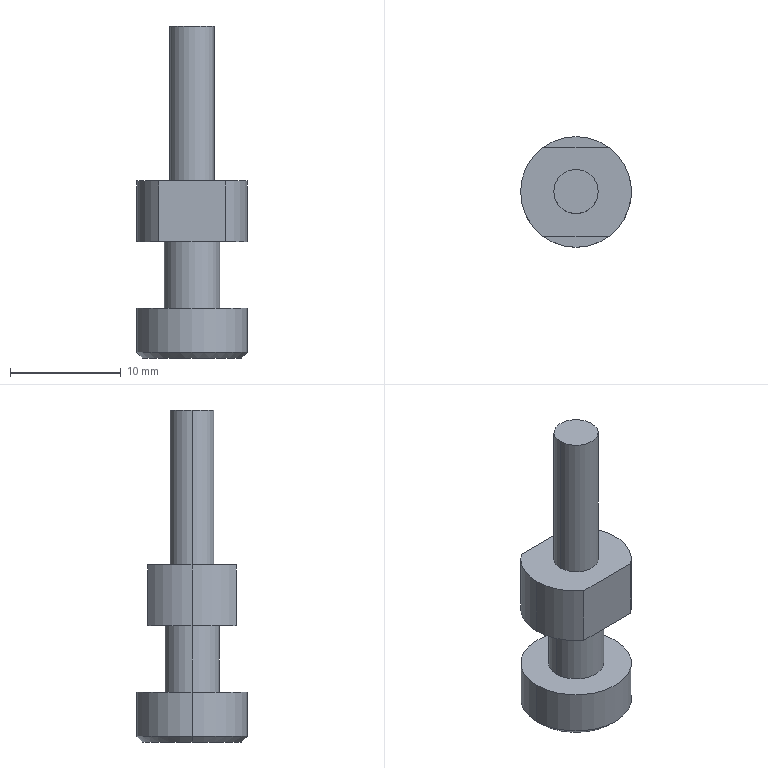Part | STEP file | PN_0008 Mount electronic clip movable head A | 1 solid | 18 faces | box 10 x 10 x 30 mm | volume 1030 mm3 | cylinder 9 | plane 7 | cone 2 | commonest cylinder face diameters 10 x5 4 x2 5 x2
STEP:
#1=CARTESIAN_POINT('',(0.,0.,0.));
#2=DIRECTION('',(0.,0.,1.));
#3=DIRECTION('',(1.,0.,0.));
#4=AXIS2_PLACEMENT_3D('',#1,#2,#3);
#5=CARTESIAN_POINT('',(-4.5,0.,-10.5));
#6=VERTEX_POINT('',#5);
#7=CARTESIAN_POINT('',(4.5,0.,-10.5));
#8=VERTEX_POINT('',#7);
#9=CARTESIAN_POINT('',(0.,0.,-10.5));
#10=DIRECTION('',(0.,0.,-1.));
#11=DIRECTION('',(-1.,0.,0.));
#12=AXIS2_PLACEMENT_3D('',#9,#10,#11);
#13=CIRCLE('',#12,4.5);
#14=CARTESIAN_POINT('',(0.,0.,-10.5));
#15=DIRECTION('',(0.,0.,1.));
#16=DIRECTION('',(1.,0.,0.));
#17=AXIS2_PLACEMENT_3D('',#14,#15,#16);
#18=CONICAL_SURFACE('',#17,4.5,0.7854);
#19=CARTESIAN_POINT('',(3.142,0.));
#20=DIRECTION('',(-1.,0.));
#21=VECTOR('',#20,1.);
#22=LINE('',#19,#21);
#23=(GEOMETRIC_REPRESENTATION_CONTEXT(2)PARAMETRIC_REPRESENTATION_CONTEXT()REPRESENTATION_CONTEXT('',''));
#24=DEFINITIONAL_REPRESENTATION('',(#22),#23);
#25=PCURVE('',#18,#24);
#26=CARTESIAN_POINT('',(0.,0.,-10.5));
#27=DIRECTION('',(0.,0.,-1.));
#28=DIRECTION('',(-1.,0.,0.));
#29=AXIS2_PLACEMENT_3D('',#26,#27,#28);
#30=PLANE('',#29);
#31=CARTESIAN_POINT('',(0.,0.));
#32=DIRECTION('',(1.,0.));
#33=AXIS2_PLACEMENT_2D('',#31,#32);
#34=CIRCLE('',#33,4.5);
#35=(GEOMETRIC_REPRESENTATION_CONTEXT(2)PARAMETRIC_REPRESENTATION_CONTEXT()REPRESENTATION_CONTEXT('',''));
#36=DEFINITIONAL_REPRESENTATION('',(#34),#35);
#37=PCURVE('',#30,#36);
#38=SURFACE_CURVE('',#13,(#25,#37),.PCURVE_S1.);
#39=EDGE_CURVE('',#6,#8,#38,.T.);
#40=ORIENTED_EDGE('',*,*,#39,.F.);
#41=CARTESIAN_POINT('',(-5.,0.,-10.));
#42=VERTEX_POINT('',#41);
#43=CARTESIAN_POINT('',(-4.5,0.,-10.5));
#44=DIRECTION('',(-0.7071,0.,0.7071));
#45=VECTOR('',#44,1.);
#46=LINE('',#43,#45);
#47=CARTESIAN_POINT('',(3.142,0.));
#48=DIRECTION('',(0.,1.));
#49=VECTOR('',#48,1.);
#50=LINE('',#47,#49);
#51=(GEOMETRIC_REPRESENTATION_CONTEXT(2)PARAMETRIC_REPRESENTATION_CONTEXT()REPRESENTATION_CONTEXT('',''));
#52=DEFINITIONAL_REPRESENTATION('',(#50),#51);
#53=PCURVE('',#18,#52);
#54=CARTESIAN_POINT('',(0.,0.,-10.5));
#55=DIRECTION('',(0.,0.,1.));
#56=DIRECTION('',(1.,0.,0.));
#57=AXIS2_PLACEMENT_3D('',#54,#55,#56);
#58=CONICAL_SURFACE('',#57,4.5,0.7854);
#59=CARTESIAN_POINT('',(3.142,0.));
#60=DIRECTION('',(0.,1.));
#61=VECTOR('',#60,1.);
#62=LINE('',#59,#61);
#63=(GEOMETRIC_REPRESENTATION_CONTEXT(2)PARAMETRIC_REPRESENTATION_CONTEXT()REPRESENTATION_CONTEXT('',''));
#64=DEFINITIONAL_REPRESENTATION('',(#62),#63);
#65=PCURVE('',#58,#64);
#66=SURFACE_CURVE('',#46,(#53,#65),.PCURVE_S1.);
#67=EDGE_CURVE('',#6,#42,#66,.T.);
#68=ORIENTED_EDGE('',*,*,#67,.T.);
#69=CARTESIAN_POINT('',(5.,0.,-10.));
#70=VERTEX_POINT('',#69);
#71=CARTESIAN_POINT('',(0.,0.,-10.));
#72=DIRECTION('',(0.,0.,1.));
#73=DIRECTION('',(-1.,0.,0.));
#74=AXIS2_PLACEMENT_3D('',#71,#72,#73);
#75=CIRCLE('',#74,5.);
#76=CARTESIAN_POINT('',(-3.142,0.5));
#77=DIRECTION('',(1.,0.));
#78=VECTOR('',#77,1.);
#79=LINE('',#76,#78);
#80=(GEOMETRIC_REPRESENTATION_CONTEXT(2)PARAMETRIC_REPRESENTATION_CONTEXT()REPRESENTATION_CONTEXT('',''));
#81=DEFINITIONAL_REPRESENTATION('',(#79),#80);
#82=PCURVE('',#18,#81);
#83=CARTESIAN_POINT('',(0.,0.,-10.5));
#84=DIRECTION('',(0.,0.,1.));
#85=DIRECTION('',(1.,0.,0.));
#86=AXIS2_PLACEMENT_3D('',#83,#84,#85);
#87=CYLINDRICAL_SURFACE('',#86,5.);
#88=CARTESIAN_POINT('',(-3.142,0.5));
#89=DIRECTION('',(1.,0.));
#90=VECTOR('',#89,1.);
#91=LINE('',#88,#90);
#92=(GEOMETRIC_REPRESENTATION_CONTEXT(2)PARAMETRIC_REPRESENTATION_CONTEXT()REPRESENTATION_CONTEXT('',''));
#93=DEFINITIONAL_REPRESENTATION('',(#91),#92);
#94=PCURVE('',#87,#93);
#95=SURFACE_CURVE('',#75,(#82,#94),.PCURVE_S1.);
#96=EDGE_CURVE('',#70,#42,#95,.T.);
#97=ORIENTED_EDGE('',*,*,#96,.F.);
#98=CARTESIAN_POINT('',(4.5,0.,-10.5));
#99=DIRECTION('',(0.7071,0.,0.7071));
#100=VECTOR('',#99,1.);
#101=LINE('',#98,#100);
#102=CARTESIAN_POINT('',(0.,0.));
#103=DIRECTION('',(0.,1.));
#104=VECTOR('',#103,1.);
#105=LINE('',#102,#104);
#106=(GEOMETRIC_REPRESENTATION_CONTEXT(2)PARAMETRIC_REPRESENTATION_CONTEXT()REPRESENTATION_CONTEXT('',''));
#107=DEFINITIONAL_REPRESENTATION('',(#105),#106);
#108=PCURVE('',#18,#107);
#109=CARTESIAN_POINT('',(6.283,0.));
#110=DIRECTION('',(0.,1.));
#111=VECTOR('',#110,1.);
#112=LINE('',#109,#111);
#113=(GEOMETRIC_REPRESENTATION_CONTEXT(2)PARAMETRIC_REPRESENTATION_CONTEXT()REPRESENTATION_CONTEXT('',''));
#114=DEFINITIONAL_REPRESENTATION('',(#112),#113);
#115=PCURVE('',#58,#114);
#116=SURFACE_CURVE('',#101,(#108,#115),.PCURVE_S1.);
#117=EDGE_CURVE('',#8,#70,#116,.T.);
#118=ORIENTED_EDGE('',*,*,#117,.F.);
#119=EDGE_LOOP('',(#40,#68,#97,#118));
#120=FACE_BOUND('',#119,.T.);
#121=ADVANCED_FACE('',(#120),#18,.T.);
#122=ORIENTED_EDGE('',*,*,#96,.T.);
#123=CARTESIAN_POINT('',(-5.,0.,-6.));
#124=VERTEX_POINT('',#123);
#125=CARTESIAN_POINT('',(-5.,0.,-10.5));
#126=DIRECTION('',(0.,0.,1.));
#127=VECTOR('',#126,1.);
#128=LINE('',#125,#127);
#129=CARTESIAN_POINT('',(3.142,0.));
#130=DIRECTION('',(0.,1.));
#131=VECTOR('',#130,1.);
#132=LINE('',#129,#131);
#133=(GEOMETRIC_REPRESENTATION_CONTEXT(2)PARAMETRIC_REPRESENTATION_CONTEXT()REPRESENTATION_CONTEXT('',''));
#134=DEFINITIONAL_REPRESENTATION('',(#132),#133);
#135=PCURVE('',#87,#134);
#136=CARTESIAN_POINT('',(0.,0.,-10.5));
#137=DIRECTION('',(0.,0.,1.));
#138=DIRECTION('',(1.,0.,0.));
#139=AXIS2_PLACEMENT_3D('',#136,#137,#138);
#140=CYLINDRICAL_SURFACE('',#139,5.);
#141=CARTESIAN_POINT('',(3.142,0.));
#142=DIRECTION('',(0.,1.));
#143=VECTOR('',#142,1.);
#144=LINE('',#141,#143);
#145=(GEOMETRIC_REPRESENTATION_CONTEXT(2)PARAMETRIC_REPRESENTATION_CONTEXT()REPRESENTATION_CONTEXT('',''));
#146=DEFINITIONAL_REPRESENTATION('',(#144),#145);
#147=PCURVE('',#140,#146);
#148=SURFACE_CURVE('',#128,(#135,#147),.PCURVE_S1.);
#149=EDGE_CURVE('',#42,#124,#148,.T.);
#150=ORIENTED_EDGE('',*,*,#149,.T.);
#151=CARTESIAN_POINT('',(5.,0.,-6.));
#152=VERTEX_POINT('',#151);
#153=CARTESIAN_POINT('',(0.,0.,-6.));
#154=DIRECTION('',(0.,0.,-1.));
#155=DIRECTION('',(-1.,0.,0.));
#156=AXIS2_PLACEMENT_3D('',#153,#154,#155);
#157=CIRCLE('',#156,5.);
#158=CARTESIAN_POINT('',(3.142,4.5));
#159=DIRECTION('',(-1.,0.));
#160=VECTOR('',#159,1.);
#161=LINE('',#158,#160);
#162=(GEOMETRIC_REPRESENTATION_CONTEXT(2)PARAMETRIC_REPRESENTATION_CONTEXT()REPRESENTATION_CONTEXT('',''));
#163=DEFINITIONAL_REPRESENTATION('',(#161),#162);
#164=PCURVE('',#87,#163);
#165=CARTESIAN_POINT('',(0.,0.,-6.));
#166=DIRECTION('',(0.,0.,-1.));
#167=DIRECTION('',(-1.,0.,0.));
#168=AXIS2_PLACEMENT_3D('',#165,#166,#167);
#169=PLANE('',#168);
#170=CARTESIAN_POINT('',(0.,0.));
#171=DIRECTION('',(1.,0.));
#172=AXIS2_PLACEMENT_2D('',#170,#171);
#173=CIRCLE('',#172,5.);
#174=(GEOMETRIC_REPRESENTATION_CONTEXT(2)PARAMETRIC_REPRESENTATION_CONTEXT()REPRESENTATION_CONTEXT('',''));
#175=DEFINITIONAL_REPRESENTATION('',(#173),#174);
#176=PCURVE('',#169,#175);
#177=SURFACE_CURVE('',#157,(#164,#176),.PCURVE_S1.);
#178=EDGE_CURVE('',#124,#152,#177,.T.);
#179=ORIENTED_EDGE('',*,*,#178,.T.);
#180=CARTESIAN_POINT('',(5.,0.,-10.5));
#181=DIRECTION('',(0.,0.,1.));
#182=VECTOR('',#181,1.);
#183=LINE('',#180,#182);
#184=CARTESIAN_POINT('',(0.,0.));
#185=DIRECTION('',(0.,1.));
#186=VECTOR('',#185,1.);
#187=LINE('',#184,#186);
#188=(GEOMETRIC_REPRESENTATION_CONTEXT(2)PARAMETRIC_REPRESENTATION_CONTEXT()REPRESENTATION_CONTEXT('',''));
#189=DEFINITIONAL_REPRESENTATION('',(#187),#188);
#190=PCURVE('',#87,#189);
#191=CARTESIAN_POINT('',(6.283,0.));
#192=DIRECTION('',(0.,1.));
#193=VECTOR('',#192,1.);
#194=LINE('',#191,#193);
#195=(GEOMETRIC_REPRESENTATION_CONTEXT(2)PARAMETRIC_REPRESENTATION_CONTEXT()REPRESENTATION_CONTEXT('',''));
#196=DEFINITIONAL_REPRESENTATION('',(#194),#195);
#197=PCURVE('',#140,#196);
#198=SURFACE_CURVE('',#183,(#190,#197),.PCURVE_S1.);
#199=EDGE_CURVE('',#70,#152,#198,.T.);
#200=ORIENTED_EDGE('',*,*,#199,.F.);
#201=EDGE_LOOP('',(#122,#150,#179,#200));
#202=FACE_BOUND('',#201,.T.);
#203=ADVANCED_FACE('',(#202),#87,.T.);
#204=CARTESIAN_POINT('',(-2.5,0.,-6.));
#205=VERTEX_POINT('',#204);
#206=CARTESIAN_POINT('',(2.5,0.,-6.));
#207=VERTEX_POINT('',#206);
#208=CARTESIAN_POINT('',(0.,0.,-6.));
#209=DIRECTION('',(0.,0.,-1.));
#210=DIRECTION('',(-1.,0.,0.));
#211=AXIS2_PLACEMENT_3D('',#208,#209,#210);
#212=CIRCLE('',#211,2.5);
#213=CARTESIAN_POINT('',(0.,0.,-6.));
#214=DIRECTION('',(0.,0.,1.));
#215=DIRECTION('',(1.,0.,0.));
#216=AXIS2_PLACEMENT_3D('',#213,#214,#215);
#217=CYLINDRICAL_SURFACE('',#216,2.5);
#218=CARTESIAN_POINT('',(3.142,0.));
#219=DIRECTION('',(-1.,0.));
#220=VECTOR('',#219,1.);
#221=LINE('',#218,#220);
#222=(GEOMETRIC_REPRESENTATION_CONTEXT(2)PARAMETRIC_REPRESENTATION_CONTEXT()REPRESENTATION_CONTEXT('',''));
#223=DEFINITIONAL_REPRESENTATION('',(#221),#222);
#224=PCURVE('',#217,#223);
#225=CARTESIAN_POINT('',(0.,0.));
#226=DIRECTION('',(1.,0.));
#227=AXIS2_PLACEMENT_2D('',#225,#226);
#228=CIRCLE('',#227,2.5);
#229=(GEOMETRIC_REPRESENTATION_CONTEXT(2)PARAMETRIC_REPRESENTATION_CONTEXT()REPRESENTATION_CONTEXT('',''));
#230=DEFINITIONAL_REPRESENTATION('',(#228),#229);
#231=PCURVE('',#169,#230);
#232=SURFACE_CURVE('',#212,(#224,#231),.PCURVE_S1.);
#233=EDGE_CURVE('',#205,#207,#232,.T.);
#234=ORIENTED_EDGE('',*,*,#233,.F.);
#235=CARTESIAN_POINT('',(-2.5,0.,0.));
#236=VERTEX_POINT('',#235);
#237=CARTESIAN_POINT('',(-2.5,0.,-6.));
#238=DIRECTION('',(0.,0.,1.));
#239=VECTOR('',#238,1.);
#240=LINE('',#237,#239);
#241=CARTESIAN_POINT('',(3.142,0.));
#242=DIRECTION('',(0.,1.));
#243=VECTOR('',#242,1.);
#244=LINE('',#241,#243);
#245=(GEOMETRIC_REPRESENTATION_CONTEXT(2)PARAMETRIC_REPRESENTATION_CONTEXT()REPRESENTATION_CONTEXT('',''));
#246=DEFINITIONAL_REPRESENTATION('',(#244),#245);
#247=PCURVE('',#217,#246);
#248=CARTESIAN_POINT('',(0.,0.,-6.));
#249=DIRECTION('',(0.,0.,1.));
#250=DIRECTION('',(1.,0.,0.));
#251=AXIS2_PLACEMENT_3D('',#248,#249,#250);
#252=CYLINDRICAL_SURFACE('',#251,2.5);
#253=CARTESIAN_POINT('',(3.142,0.));
#254=DIRECTION('',(0.,1.));
#255=VECTOR('',#254,1.);
#256=LINE('',#253,#255);
#257=(GEOMETRIC_REPRESENTATION_CONTEXT(2)PARAMETRIC_REPRESENTATION_CONTEXT()REPRESENTATION_CONTEXT('',''));
#258=DEFINITIONAL_REPRESENTATION('',(#256),#257);
#259=PCURVE('',#252,#258);
#260=SURFACE_CURVE('',#240,(#247,#259),.PCURVE_S1.);
#261=EDGE_CURVE('',#205,#236,#260,.T.);
#262=ORIENTED_EDGE('',*,*,#261,.T.);
#263=CARTESIAN_POINT('',(2.5,0.,0.));
#264=VERTEX_POINT('',#263);
#265=CARTESIAN_POINT('',(0.,0.,0.));
#266=DIRECTION('',(0.,0.,-1.));
#267=DIRECTION('',(1.,0.,0.));
#268=AXIS2_PLACEMENT_3D('',#265,#266,#267);
#269=CIRCLE('',#268,2.5);
#270=CARTESIAN_POINT('',(6.283,6.));
#271=DIRECTION('',(-1.,0.));
#272=VECTOR('',#271,1.);
#273=LINE('',#270,#272);
#274=(GEOMETRIC_REPRESENTATION_CONTEXT(2)PARAMETRIC_REPRESENTATION_CONTEXT()REPRESENTATION_CONTEXT('',''));
#275=DEFINITIONAL_REPRESENTATION('',(#273),#274);
#276=PCURVE('',#217,#275);
#277=CARTESIAN_POINT('',(0.,0.,0.));
#278=DIRECTION('',(0.,0.,1.));
#279=DIRECTION('',(1.,0.,0.));
#280=AXIS2_PLACEMENT_3D('',#277,#278,#279);
#281=PLANE('',#280);
#282=CARTESIAN_POINT('',(2.5,0.));
#283=CARTESIAN_POINT('',(2.5,-4.33));
#284=CARTESIAN_POINT('',(-1.25,-2.165));
#285=CARTESIAN_POINT('',(-5.,0.));
#286=CARTESIAN_POINT('',(-1.25,2.165));
#287=CARTESIAN_POINT('',(2.5,4.33));
#288=CARTESIAN_POINT('',(2.5,0.));
#289=(BOUNDED_CURVE()B_SPLINE_CURVE(2,(#282,#283,#284,#285,#286,#287,#288),.UNSPECIFIED.,.T.,.F.)B_SPLINE_CURVE_WITH_KNOTS((1,2,2,2,2,1),(-2.094,0.,2.094,4.189,6.283,8.378),.UNSPECIFIED.)CURVE()GEOMETRIC_REPRESENTATION_ITEM()RATIONAL_B_SPLINE_CURVE((1.,0.5,1.,0.5,1.,0.5,1.))REPRESENTATION_ITEM(''));
#290=(GEOMETRIC_REPRESENTATION_CONTEXT(2)PARAMETRIC_REPRESENTATION_CONTEXT()REPRESENTATION_CONTEXT('',''));
#291=DEFINITIONAL_REPRESENTATION('',(#289),#290);
#292=PCURVE('',#281,#291);
#293=SURFACE_CURVE('',#269,(#276,#292),.PCURVE_S1.);
#294=EDGE_CURVE('',#236,#264,#293,.T.);
#295=ORIENTED_EDGE('',*,*,#294,.T.);
#296=CARTESIAN_POINT('',(2.5,0.,-6.));
#297=DIRECTION('',(0.,0.,1.));
#298=VECTOR('',#297,1.);
#299=LINE('',#296,#298);
#300=CARTESIAN_POINT('',(0.,0.));
#301=DIRECTION('',(0.,1.));
#302=VECTOR('',#301,1.);
#303=LINE('',#300,#302);
#304=(GEOMETRIC_REPRESENTATION_CONTEXT(2)PARAMETRIC_REPRESENTATION_CONTEXT()REPRESENTATION_CONTEXT('',''));
#305=DEFINITIONAL_REPRESENTATION('',(#303),#304);
#306=PCURVE('',#217,#305);
#307=CARTESIAN_POINT('',(6.283,0.));
#308=DIRECTION('',(0.,1.));
#309=VECTOR('',#308,1.);
#310=LINE('',#307,#309);
#311=(GEOMETRIC_REPRESENTATION_CONTEXT(2)PARAMETRIC_REPRESENTATION_CONTEXT()REPRESENTATION_CONTEXT('',''));
#312=DEFINITIONAL_REPRESENTATION('',(#310),#311);
#313=PCURVE('',#252,#312);
#314=SURFACE_CURVE('',#299,(#306,#313),.PCURVE_S1.);
#315=EDGE_CURVE('',#207,#264,#314,.T.);
#316=ORIENTED_EDGE('',*,*,#315,.F.);
#317=EDGE_LOOP('',(#234,#262,#295,#316));
#318=FACE_BOUND('',#317,.T.);
#319=ADVANCED_FACE('',(#318),#217,.T.);
#320=CARTESIAN_POINT('',(2.,0.,19.5));
#321=VERTEX_POINT('',#320);
#322=CARTESIAN_POINT('',(-2.,0.,19.5));
#323=VERTEX_POINT('',#322);
#324=CARTESIAN_POINT('',(0.,0.,19.5));
#325=DIRECTION('',(0.,0.,1.));
#326=DIRECTION('',(1.,0.,0.));
#327=AXIS2_PLACEMENT_3D('',#324,#325,#326);
#328=CIRCLE('',#327,2.);
#329=CARTESIAN_POINT('',(0.,0.,19.5));
#330=DIRECTION('',(0.,0.,-1.));
#331=DIRECTION('',(-1.,0.,0.));
#332=AXIS2_PLACEMENT_3D('',#329,#330,#331);
#333=CYLINDRICAL_SURFACE('',#332,2.);
#334=CARTESIAN_POINT('',(3.142,0.));
#335=DIRECTION('',(-1.,0.));
#336=VECTOR('',#335,1.);
#337=LINE('',#334,#336);
#338=(GEOMETRIC_REPRESENTATION_CONTEXT(2)PARAMETRIC_REPRESENTATION_CONTEXT()REPRESENTATION_CONTEXT('',''));
#339=DEFINITIONAL_REPRESENTATION('',(#337),#338);
#340=PCURVE('',#333,#339);
#341=CARTESIAN_POINT('',(0.,0.,19.5));
#342=DIRECTION('',(0.,0.,1.));
#343=DIRECTION('',(1.,0.,0.));
#344=AXIS2_PLACEMENT_3D('',#341,#342,#343);
#345=PLANE('',#344);
#346=CARTESIAN_POINT('',(0.,0.));
#347=DIRECTION('',(1.,0.));
#348=AXIS2_PLACEMENT_2D('',#346,#347);
#349=CIRCLE('',#348,2.);
#350=(GEOMETRIC_REPRESENTATION_CONTEXT(2)PARAMETRIC_REPRESENTATION_CONTEXT()REPRESENTATION_CONTEXT('',''));
#351=DEFINITIONAL_REPRESENTATION('',(#349),#350);
#352=PCURVE('',#345,#351);
#353=SURFACE_CURVE('',#328,(#340,#352),.PCURVE_S1.);
#354=EDGE_CURVE('',#321,#323,#353,.T.);
#355=ORIENTED_EDGE('',*,*,#354,.F.);
#356=CARTESIAN_POINT('',(2.,0.,5.5));
#357=VERTEX_POINT('',#356);
#358=CARTESIAN_POINT('',(2.,0.,19.5));
#359=DIRECTION('',(0.,0.,-1.));
#360=VECTOR('',#359,1.);
#361=LINE('',#358,#360);
#362=CARTESIAN_POINT('',(3.142,0.));
#363=DIRECTION('',(0.,1.));
#364=VECTOR('',#363,1.);
#365=LINE('',#362,#364);
#366=(GEOMETRIC_REPRESENTATION_CONTEXT(2)PARAMETRIC_REPRESENTATION_CONTEXT()REPRESENTATION_CONTEXT('',''));
#367=DEFINITIONAL_REPRESENTATION('',(#365),#366);
#368=PCURVE('',#333,#367);
#369=CARTESIAN_POINT('',(0.,0.,19.5));
#370=DIRECTION('',(0.,0.,-1.));
#371=DIRECTION('',(-1.,0.,0.));
#372=AXIS2_PLACEMENT_3D('',#369,#370,#371);
#373=CYLINDRICAL_SURFACE('',#372,2.);
#374=CARTESIAN_POINT('',(3.142,0.));
#375=DIRECTION('',(0.,1.));
#376=VECTOR('',#375,1.);
#377=LINE('',#374,#376);
#378=(GEOMETRIC_REPRESENTATION_CONTEXT(2)PARAMETRIC_REPRESENTATION_CONTEXT()REPRESENTATION_CONTEXT('',''));
#379=DEFINITIONAL_REPRESENTATION('',(#377),#378);
#380=PCURVE('',#373,#379);
#381=SURFACE_CURVE('',#361,(#368,#380),.PCURVE_S1.);
#382=EDGE_CURVE('',#321,#357,#381,.T.);
#383=ORIENTED_EDGE('',*,*,#382,.T.);
#384=CARTESIAN_POINT('',(-2.,0.,5.5));
#385=VERTEX_POINT('',#384);
#386=CARTESIAN_POINT('',(0.,0.,5.5));
#387=DIRECTION('',(0.,0.,1.));
#388=DIRECTION('',(1.,0.,0.));
#389=AXIS2_PLACEMENT_3D('',#386,#387,#388);
#390=CIRCLE('',#389,2.);
#391=CARTESIAN_POINT('',(3.142,14.));
#392=DIRECTION('',(-1.,0.));
#393=VECTOR('',#392,1.);
#394=LINE('',#391,#393);
#395=(GEOMETRIC_REPRESENTATION_CONTEXT(2)PARAMETRIC_REPRESENTATION_CONTEXT()REPRESENTATION_CONTEXT('',''));
#396=DEFINITIONAL_REPRESENTATION('',(#394),#395);
#397=PCURVE('',#333,#396);
#398=CARTESIAN_POINT('',(0.,0.,5.5));
#399=DIRECTION('',(0.,0.,1.));
#400=DIRECTION('',(1.,0.,0.));
#401=AXIS2_PLACEMENT_3D('',#398,#399,#400);
#402=PLANE('',#401);
#403=CARTESIAN_POINT('',(0.,0.));
#404=DIRECTION('',(1.,0.));
#405=AXIS2_PLACEMENT_2D('',#403,#404);
#406=CIRCLE('',#405,2.);
#407=(GEOMETRIC_REPRESENTATION_CONTEXT(2)PARAMETRIC_REPRESENTATION_CONTEXT()REPRESENTATION_CONTEXT('',''));
#408=DEFINITIONAL_REPRESENTATION('',(#406),#407);
#409=PCURVE('',#402,#408);
#410=SURFACE_CURVE('',#390,(#397,#409),.PCURVE_S1.);
#411=EDGE_CURVE('',#357,#385,#410,.T.);
#412=ORIENTED_EDGE('',*,*,#411,.T.);
#413=CARTESIAN_POINT('',(-2.,0.,19.5));
#414=DIRECTION('',(0.,0.,-1.));
#415=VECTOR('',#414,1.);
#416=LINE('',#413,#415);
#417=CARTESIAN_POINT('',(0.,0.));
#418=DIRECTION('',(0.,1.));
#419=VECTOR('',#418,1.);
#420=LINE('',#417,#419);
#421=(GEOMETRIC_REPRESENTATION_CONTEXT(2)PARAMETRIC_REPRESENTATION_CONTEXT()REPRESENTATION_CONTEXT('',''));
#422=DEFINITIONAL_REPRESENTATION('',(#420),#421);
#423=PCURVE('',#333,#422);
#424=CARTESIAN_POINT('',(6.283,0.));
#425=DIRECTION('',(0.,1.));
#426=VECTOR('',#425,1.);
#427=LINE('',#424,#426);
#428=(GEOMETRIC_REPRESENTATION_CONTEXT(2)PARAMETRIC_REPRESENTATION_CONTEXT()REPRESENTATION_CONTEXT('',''));
#429=DEFINITIONAL_REPRESENTATION('',(#427),#428);
#430=PCURVE('',#373,#429);
#431=SURFACE_CURVE('',#416,(#423,#430),.PCURVE_S1.);
#432=EDGE_CURVE('',#323,#385,#431,.T.);
#433=ORIENTED_EDGE('',*,*,#432,.F.);
#434=EDGE_LOOP('',(#355,#383,#412,#433));
#435=FACE_BOUND('',#434,.T.);
#436=ADVANCED_FACE('',(#435),#333,.T.);
#437=CARTESIAN_POINT('',(-5.,0.,5.5));
#438=VERTEX_POINT('',#437);
#439=CARTESIAN_POINT('',(-3.,-4.,5.5));
#440=VERTEX_POINT('',#439);
#441=CARTESIAN_POINT('',(0.,0.,5.5));
#442=DIRECTION('',(0.,0.,1.));
#443=DIRECTION('',(1.,0.,0.));
#444=AXIS2_PLACEMENT_3D('',#441,#442,#443);
#445=CIRCLE('',#444,5.);
#446=CARTESIAN_POINT('',(0.,0.,5.5));
#447=DIRECTION('',(0.,0.,-1.));
#448=DIRECTION('',(-1.,0.,0.));
#449=AXIS2_PLACEMENT_3D('',#446,#447,#448);
#450=CYLINDRICAL_SURFACE('',#449,5.);
#451=CARTESIAN_POINT('',(9.425,0.));
#452=DIRECTION('',(-1.,0.));
#453=VECTOR('',#452,1.);
#454=LINE('',#451,#453);
#455=(GEOMETRIC_REPRESENTATION_CONTEXT(2)PARAMETRIC_REPRESENTATION_CONTEXT()REPRESENTATION_CONTEXT('',''));
#456=DEFINITIONAL_REPRESENTATION('',(#454),#455);
#457=PCURVE('',#450,#456);
#458=CARTESIAN_POINT('',(0.,0.));
#459=DIRECTION('',(1.,0.));
#460=AXIS2_PLACEMENT_2D('',#458,#459);
#461=CIRCLE('',#460,5.);
#462=(GEOMETRIC_REPRESENTATION_CONTEXT(2)PARAMETRIC_REPRESENTATION_CONTEXT()REPRESENTATION_CONTEXT('',''));
#463=DEFINITIONAL_REPRESENTATION('',(#461),#462);
#464=PCURVE('',#402,#463);
#465=SURFACE_CURVE('',#445,(#457,#464),.PCURVE_S1.);
#466=EDGE_CURVE('',#438,#440,#465,.T.);
#467=ORIENTED_EDGE('',*,*,#466,.F.);
#468=CARTESIAN_POINT('',(-5.,0.,0.));
#469=VERTEX_POINT('',#468);
#470=CARTESIAN_POINT('',(-5.,0.,5.5));
#471=DIRECTION('',(0.,0.,-1.));
#472=VECTOR('',#471,1.);
#473=LINE('',#470,#472);
#474=CARTESIAN_POINT('',(6.283,0.));
#475=DIRECTION('',(0.,1.));
#476=VECTOR('',#475,1.);
#477=LINE('',#474,#476);
#478=(GEOMETRIC_REPRESENTATION_CONTEXT(2)PARAMETRIC_REPRESENTATION_CONTEXT()REPRESENTATION_CONTEXT('',''));
#479=DEFINITIONAL_REPRESENTATION('',(#477),#478);
#480=PCURVE('',#450,#479);
#481=CARTESIAN_POINT('',(0.,0.,5.5));
#482=DIRECTION('',(0.,0.,-1.));
#483=DIRECTION('',(-1.,0.,0.));
#484=AXIS2_PLACEMENT_3D('',#481,#482,#483);
#485=CYLINDRICAL_SURFACE('',#484,5.);
#486=CARTESIAN_POINT('',(0.,0.));
#487=DIRECTION('',(0.,1.));
#488=VECTOR('',#487,1.);
#489=LINE('',#486,#488);
#490=(GEOMETRIC_REPRESENTATION_CONTEXT(2)PARAMETRIC_REPRESENTATION_CONTEXT()REPRESENTATION_CONTEXT('',''));
#491=DEFINITIONAL_REPRESENTATION('',(#489),#490);
#492=PCURVE('',#485,#491);
#493=SURFACE_CURVE('',#473,(#480,#492),.PCURVE_S1.);
#494=EDGE_CURVE('',#438,#469,#493,.T.);
#495=ORIENTED_EDGE('',*,*,#494,.T.);
#496=CARTESIAN_POINT('',(-3.,-4.,0.));
#497=VERTEX_POINT('',#496);
#498=CARTESIAN_POINT('',(0.,0.,0.));
#499=DIRECTION('',(0.,0.,1.));
#500=DIRECTION('',(1.,0.,0.));
#501=AXIS2_PLACEMENT_3D('',#498,#499,#500);
#502=CIRCLE('',#501,5.);
#503=CARTESIAN_POINT('',(9.425,5.5));
#504=DIRECTION('',(-1.,0.));
#505=VECTOR('',#504,1.);
#506=LINE('',#503,#505);
#507=(GEOMETRIC_REPRESENTATION_CONTEXT(2)PARAMETRIC_REPRESENTATION_CONTEXT()REPRESENTATION_CONTEXT('',''));
#508=DEFINITIONAL_REPRESENTATION('',(#506),#507);
#509=PCURVE('',#450,#508);
#510=CARTESIAN_POINT('',(0.,0.));
#511=DIRECTION('',(1.,0.));
#512=AXIS2_PLACEMENT_2D('',#510,#511);
#513=CIRCLE('',#512,5.);
#514=(GEOMETRIC_REPRESENTATION_CONTEXT(2)PARAMETRIC_REPRESENTATION_CONTEXT()REPRESENTATION_CONTEXT('',''));
#515=DEFINITIONAL_REPRESENTATION('',(#513),#514);
#516=PCURVE('',#281,#515);
#517=SURFACE_CURVE('',#502,(#509,#516),.PCURVE_S1.);
#518=EDGE_CURVE('',#469,#497,#517,.T.);
#519=ORIENTED_EDGE('',*,*,#518,.T.);
#520=CARTESIAN_POINT('',(-3.,-4.,5.5));
#521=DIRECTION('',(0.,0.,-1.));
#522=VECTOR('',#521,1.);
#523=LINE('',#520,#522);
#524=CARTESIAN_POINT('',(5.356,0.));
#525=DIRECTION('',(0.,1.));
#526=VECTOR('',#525,1.);
#527=LINE('',#524,#526);
#528=(GEOMETRIC_REPRESENTATION_CONTEXT(2)PARAMETRIC_REPRESENTATION_CONTEXT()REPRESENTATION_CONTEXT('',''));
#529=DEFINITIONAL_REPRESENTATION('',(#527),#528);
#530=PCURVE('',#450,#529);
#531=CARTESIAN_POINT('',(7.775,-4.,10.));
#532=DIRECTION('',(0.,-1.,0.));
#533=DIRECTION('',(0.,0.,-1.));
#534=AXIS2_PLACEMENT_3D('',#531,#532,#533);
#535=PLANE('',#534);
#536=CARTESIAN_POINT('',(4.5,-10.775));
#537=DIRECTION('',(1.,0.));
#538=VECTOR('',#537,1.);
#539=LINE('',#536,#538);
#540=(GEOMETRIC_REPRESENTATION_CONTEXT(2)PARAMETRIC_REPRESENTATION_CONTEXT()REPRESENTATION_CONTEXT('',''));
#541=DEFINITIONAL_REPRESENTATION('',(#539),#540);
#542=PCURVE('',#535,#541);
#543=SURFACE_CURVE('',#523,(#530,#542),.PCURVE_S1.);
#544=EDGE_CURVE('',#440,#497,#543,.T.);
#545=ORIENTED_EDGE('',*,*,#544,.F.);
#546=EDGE_LOOP('',(#467,#495,#519,#545));
#547=FACE_BOUND('',#546,.T.);
#548=ADVANCED_FACE('',(#547),#450,.T.);
#549=CARTESIAN_POINT('',(3.,-4.,0.));
#550=VERTEX_POINT('',#549);
#551=CARTESIAN_POINT('',(0.,-4.,0.));
#552=DIRECTION('',(1.,0.,0.));
#553=VECTOR('',#552,1.);
#554=LINE('',#551,#553);
#555=CARTESIAN_POINT('',(0.,-4.));
#556=DIRECTION('',(1.,0.));
#557=VECTOR('',#556,1.);
#558=LINE('',#555,#557);
#559=(GEOMETRIC_REPRESENTATION_CONTEXT(2)PARAMETRIC_REPRESENTATION_CONTEXT()REPRESENTATION_CONTEXT('',''));
#560=DEFINITIONAL_REPRESENTATION('',(#558),#559);
#561=PCURVE('',#281,#560);
#562=CARTESIAN_POINT('',(10.,-7.775));
#563=DIRECTION('',(0.,1.));
#564=VECTOR('',#563,1.);
#565=LINE('',#562,#564);
#566=(GEOMETRIC_REPRESENTATION_CONTEXT(2)PARAMETRIC_REPRESENTATION_CONTEXT()REPRESENTATION_CONTEXT('',''));
#567=DEFINITIONAL_REPRESENTATION('',(#565),#566);
#568=PCURVE('',#535,#567);
#569=SURFACE_CURVE('',#554,(#561,#568),.PCURVE_S1.);
#570=EDGE_CURVE('',#497,#550,#569,.T.);
#571=ORIENTED_EDGE('',*,*,#570,.F.);
#572=ORIENTED_EDGE('',*,*,#518,.F.);
#573=CARTESIAN_POINT('',(-3.,4.,0.));
#574=VERTEX_POINT('',#573);
#575=CARTESIAN_POINT('',(0.,0.,0.));
#576=DIRECTION('',(0.,0.,1.));
#577=DIRECTION('',(1.,0.,0.));
#578=AXIS2_PLACEMENT_3D('',#575,#576,#577);
#579=CIRCLE('',#578,5.);
#580=CARTESIAN_POINT('',(0.,0.));
#581=DIRECTION('',(1.,0.));
#582=AXIS2_PLACEMENT_2D('',#580,#581);
#583=CIRCLE('',#582,5.);
#584=(GEOMETRIC_REPRESENTATION_CONTEXT(2)PARAMETRIC_REPRESENTATION_CONTEXT()REPRESENTATION_CONTEXT('',''));
#585=DEFINITIONAL_REPRESENTATION('',(#583),#584);
#586=PCURVE('',#281,#585);
#587=CARTESIAN_POINT('',(3.142,5.5));
#588=DIRECTION('',(-1.,0.));
#589=VECTOR('',#588,1.);
#590=LINE('',#587,#589);
#591=(GEOMETRIC_REPRESENTATION_CONTEXT(2)PARAMETRIC_REPRESENTATION_CONTEXT()REPRESENTATION_CONTEXT('',''));
#592=DEFINITIONAL_REPRESENTATION('',(#590),#591);
#593=PCURVE('',#485,#592);
#594=SURFACE_CURVE('',#579,(#586,#593),.PCURVE_S1.);
#595=EDGE_CURVE('',#574,#469,#594,.T.);
#596=ORIENTED_EDGE('',*,*,#595,.F.);
#597=CARTESIAN_POINT('',(3.,4.,0.));
#598=VERTEX_POINT('',#597);
#599=CARTESIAN_POINT('',(0.,4.,0.));
#600=DIRECTION('',(-1.,0.,0.));
#601=VECTOR('',#600,1.);
#602=LINE('',#599,#601);
#603=CARTESIAN_POINT('',(0.,4.));
#604=DIRECTION('',(-1.,0.));
#605=VECTOR('',#604,1.);
#606=LINE('',#603,#605);
#607=(GEOMETRIC_REPRESENTATION_CONTEXT(2)PARAMETRIC_REPRESENTATION_CONTEXT()REPRESENTATION_CONTEXT('',''));
#608=DEFINITIONAL_REPRESENTATION('',(#606),#607);
#609=PCURVE('',#281,#608);
#610=CARTESIAN_POINT('',(7.775,4.,10.));
#611=DIRECTION('',(0.,1.,0.));
#612=DIRECTION('',(0.,0.,1.));
#613=AXIS2_PLACEMENT_3D('',#610,#611,#612);
#614=PLANE('',#613);
#615=CARTESIAN_POINT('',(-10.,-7.775));
#616=DIRECTION('',(0.,-1.));
#617=VECTOR('',#616,1.);
#618=LINE('',#615,#617);
#619=(GEOMETRIC_REPRESENTATION_CONTEXT(2)PARAMETRIC_REPRESENTATION_CONTEXT()REPRESENTATION_CONTEXT('',''));
#620=DEFINITIONAL_REPRESENTATION('',(#618),#619);
#621=PCURVE('',#614,#620);
#622=SURFACE_CURVE('',#602,(#609,#621),.PCURVE_S1.);
#623=EDGE_CURVE('',#598,#574,#622,.T.);
#624=ORIENTED_EDGE('',*,*,#623,.F.);
#625=CARTESIAN_POINT('',(0.,0.,0.));
#626=DIRECTION('',(0.,0.,1.));
#627=DIRECTION('',(1.,0.,0.));
#628=AXIS2_PLACEMENT_3D('',#625,#626,#627);
#629=CIRCLE('',#628,5.);
#630=CARTESIAN_POINT('',(0.,0.));
#631=DIRECTION('',(1.,0.));
#632=AXIS2_PLACEMENT_2D('',#630,#631);
#633=CIRCLE('',#632,5.);
#634=(GEOMETRIC_REPRESENTATION_CONTEXT(2)PARAMETRIC_REPRESENTATION_CONTEXT()REPRESENTATION_CONTEXT('',''));
#635=DEFINITIONAL_REPRESENTATION('',(#633),#634);
#636=PCURVE('',#281,#635);
#637=CARTESIAN_POINT('',(0.,0.,5.5));
#638=DIRECTION('',(0.,0.,-1.));
#639=DIRECTION('',(-1.,0.,0.));
#640=AXIS2_PLACEMENT_3D('',#637,#638,#639);
#641=CYLINDRICAL_SURFACE('',#640,5.);
#642=CARTESIAN_POINT('',(9.425,5.5));
#643=DIRECTION('',(-1.,0.));
#644=VECTOR('',#643,1.);
#645=LINE('',#642,#644);
#646=(GEOMETRIC_REPRESENTATION_CONTEXT(2)PARAMETRIC_REPRESENTATION_CONTEXT()REPRESENTATION_CONTEXT('',''));
#647=DEFINITIONAL_REPRESENTATION('',(#645),#646);
#648=PCURVE('',#641,#647);
#649=SURFACE_CURVE('',#629,(#636,#648),.PCURVE_S1.);
#650=EDGE_CURVE('',#550,#598,#649,.T.);
#651=ORIENTED_EDGE('',*,*,#650,.F.);
#652=EDGE_LOOP('',(#571,#572,#596,#624,#651));
#653=FACE_BOUND('',#652,.T.);
#654=CARTESIAN_POINT('',(0.,0.,0.));
#655=DIRECTION('',(0.,0.,-1.));
#656=DIRECTION('',(1.,0.,0.));
#657=AXIS2_PLACEMENT_3D('',#654,#655,#656);
#658=CIRCLE('',#657,2.5);
#659=CARTESIAN_POINT('',(2.5,0.));
#660=CARTESIAN_POINT('',(2.5,-4.33));
#661=CARTESIAN_POINT('',(-1.25,-2.165));
#662=CARTESIAN_POINT('',(-5.,0.));
#663=CARTESIAN_POINT('',(-1.25,2.165));
#664=CARTESIAN_POINT('',(2.5,4.33));
#665=CARTESIAN_POINT('',(2.5,0.));
#666=(BOUNDED_CURVE()B_SPLINE_CURVE(2,(#659,#660,#661,#662,#663,#664,#665),.UNSPECIFIED.,.T.,.F.)B_SPLINE_CURVE_WITH_KNOTS((1,2,2,2,2,1),(-2.094,0.,2.094,4.189,6.283,8.378),.UNSPECIFIED.)CURVE()GEOMETRIC_REPRESENTATION_ITEM()RATIONAL_B_SPLINE_CURVE((1.,0.5,1.,0.5,1.,0.5,1.))REPRESENTATION_ITEM(''));
#667=(GEOMETRIC_REPRESENTATION_CONTEXT(2)PARAMETRIC_REPRESENTATION_CONTEXT()REPRESENTATION_CONTEXT('',''));
#668=DEFINITIONAL_REPRESENTATION('',(#666),#667);
#669=PCURVE('',#281,#668);
#670=CARTESIAN_POINT('',(6.283,6.));
#671=DIRECTION('',(-1.,0.));
#672=VECTOR('',#671,1.);
#673=LINE('',#670,#672);
#674=(GEOMETRIC_REPRESENTATION_CONTEXT(2)PARAMETRIC_REPRESENTATION_CONTEXT()REPRESENTATION_CONTEXT('',''));
#675=DEFINITIONAL_REPRESENTATION('',(#673),#674);
#676=PCURVE('',#252,#675);
#677=SURFACE_CURVE('',#658,(#669,#676),.PCURVE_S1.);
#678=EDGE_CURVE('',#264,#236,#677,.T.);
#679=ORIENTED_EDGE('',*,*,#678,.F.);
#680=ORIENTED_EDGE('',*,*,#294,.F.);
#681=EDGE_LOOP('',(#679,#680));
#682=FACE_BOUND('',#681,.T.);
#683=ADVANCED_FACE('',(#653,#682),#281,.F.);
#684=CARTESIAN_POINT('',(0.,0.,5.5));
#685=DIRECTION('',(0.,0.,1.));
#686=DIRECTION('',(1.,0.,0.));
#687=AXIS2_PLACEMENT_3D('',#684,#685,#686);
#688=CIRCLE('',#687,2.);
#689=CARTESIAN_POINT('',(0.,0.));
#690=DIRECTION('',(1.,0.));
#691=AXIS2_PLACEMENT_2D('',#689,#690);
#692=CIRCLE('',#691,2.);
#693=(GEOMETRIC_REPRESENTATION_CONTEXT(2)PARAMETRIC_REPRESENTATION_CONTEXT()REPRESENTATION_CONTEXT('',''));
#694=DEFINITIONAL_REPRESENTATION('',(#692),#693);
#695=PCURVE('',#402,#694);
#696=CARTESIAN_POINT('',(9.425,14.));
#697=DIRECTION('',(-1.,0.));
#698=VECTOR('',#697,1.);
#699=LINE('',#696,#698);
#700=(GEOMETRIC_REPRESENTATION_CONTEXT(2)PARAMETRIC_REPRESENTATION_CONTEXT()REPRESENTATION_CONTEXT('',''));
#701=DEFINITIONAL_REPRESENTATION('',(#699),#700);
#702=PCURVE('',#373,#701);
#703=SURFACE_CURVE('',#688,(#695,#702),.PCURVE_S1.);
#704=EDGE_CURVE('',#385,#357,#703,.T.);
#705=ORIENTED_EDGE('',*,*,#704,.F.);
#706=ORIENTED_EDGE('',*,*,#411,.F.);
#707=EDGE_LOOP('',(#705,#706));
#708=FACE_BOUND('',#707,.T.);
#709=CARTESIAN_POINT('',(-3.,4.,5.5));
#710=VERTEX_POINT('',#709);
#711=CARTESIAN_POINT('',(0.,0.,5.5));
#712=DIRECTION('',(0.,0.,1.));
#713=DIRECTION('',(1.,0.,0.));
#714=AXIS2_PLACEMENT_3D('',#711,#712,#713);
#715=CIRCLE('',#714,5.);
#716=CARTESIAN_POINT('',(0.,0.));
#717=DIRECTION('',(1.,0.));
#718=AXIS2_PLACEMENT_2D('',#716,#717);
#719=CIRCLE('',#718,5.);
#720=(GEOMETRIC_REPRESENTATION_CONTEXT(2)PARAMETRIC_REPRESENTATION_CONTEXT()REPRESENTATION_CONTEXT('',''));
#721=DEFINITIONAL_REPRESENTATION('',(#719),#720);
#722=PCURVE('',#402,#721);
#723=CARTESIAN_POINT('',(3.142,0.));
#724=DIRECTION('',(-1.,0.));
#725=VECTOR('',#724,1.);
#726=LINE('',#723,#725);
#727=(GEOMETRIC_REPRESENTATION_CONTEXT(2)PARAMETRIC_REPRESENTATION_CONTEXT()REPRESENTATION_CONTEXT('',''));
#728=DEFINITIONAL_REPRESENTATION('',(#726),#727);
#729=PCURVE('',#485,#728);
#730=SURFACE_CURVE('',#715,(#722,#729),.PCURVE_S1.);
#731=EDGE_CURVE('',#710,#438,#730,.T.);
#732=ORIENTED_EDGE('',*,*,#731,.T.);
#733=ORIENTED_EDGE('',*,*,#466,.T.);
#734=CARTESIAN_POINT('',(3.,-4.,5.5));
#735=VERTEX_POINT('',#734);
#736=CARTESIAN_POINT('',(0.,-4.,5.5));
#737=DIRECTION('',(1.,0.,0.));
#738=VECTOR('',#737,1.);
#739=LINE('',#736,#738);
#740=CARTESIAN_POINT('',(0.,-4.));
#741=DIRECTION('',(1.,0.));
#742=VECTOR('',#741,1.);
#743=LINE('',#740,#742);
#744=(GEOMETRIC_REPRESENTATION_CONTEXT(2)PARAMETRIC_REPRESENTATION_CONTEXT()REPRESENTATION_CONTEXT('',''));
#745=DEFINITIONAL_REPRESENTATION('',(#743),#744);
#746=PCURVE('',#402,#745);
#747=CARTESIAN_POINT('',(4.5,-7.775));
#748=DIRECTION('',(0.,1.));
#749=VECTOR('',#748,1.);
#750=LINE('',#747,#749);
#751=(GEOMETRIC_REPRESENTATION_CONTEXT(2)PARAMETRIC_REPRESENTATION_CONTEXT()REPRESENTATION_CONTEXT('',''));
#752=DEFINITIONAL_REPRESENTATION('',(#750),#751);
#753=PCURVE('',#535,#752);
#754=SURFACE_CURVE('',#739,(#746,#753),.PCURVE_S1.);
#755=EDGE_CURVE('',#440,#735,#754,.T.);
#756=ORIENTED_EDGE('',*,*,#755,.T.);
#757=CARTESIAN_POINT('',(3.,4.,5.5));
#758=VERTEX_POINT('',#757);
#759=CARTESIAN_POINT('',(0.,0.,5.5));
#760=DIRECTION('',(0.,0.,1.));
#761=DIRECTION('',(1.,0.,0.));
#762=AXIS2_PLACEMENT_3D('',#759,#760,#761);
#763=CIRCLE('',#762,5.);
#764=CARTESIAN_POINT('',(0.,0.));
#765=DIRECTION('',(1.,0.));
#766=AXIS2_PLACEMENT_2D('',#764,#765);
#767=CIRCLE('',#766,5.);
#768=(GEOMETRIC_REPRESENTATION_CONTEXT(2)PARAMETRIC_REPRESENTATION_CONTEXT()REPRESENTATION_CONTEXT('',''));
#769=DEFINITIONAL_REPRESENTATION('',(#767),#768);
#770=PCURVE('',#402,#769);
#771=CARTESIAN_POINT('',(9.425,0.));
#772=DIRECTION('',(-1.,0.));
#773=VECTOR('',#772,1.);
#774=LINE('',#771,#773);
#775=(GEOMETRIC_REPRESENTATION_CONTEXT(2)PARAMETRIC_REPRESENTATION_CONTEXT()REPRESENTATION_CONTEXT('',''));
#776=DEFINITIONAL_REPRESENTATION('',(#774),#775);
#777=PCURVE('',#641,#776);
#778=SURFACE_CURVE('',#763,(#770,#777),.PCURVE_S1.);
#779=EDGE_CURVE('',#735,#758,#778,.T.);
#780=ORIENTED_EDGE('',*,*,#779,.T.);
#781=CARTESIAN_POINT('',(0.,4.,5.5));
#782=DIRECTION('',(-1.,0.,0.));
#783=VECTOR('',#782,1.);
#784=LINE('',#781,#783);
#785=CARTESIAN_POINT('',(0.,4.));
#786=DIRECTION('',(-1.,0.));
#787=VECTOR('',#786,1.);
#788=LINE('',#785,#787);
#789=(GEOMETRIC_REPRESENTATION_CONTEXT(2)PARAMETRIC_REPRESENTATION_CONTEXT()REPRESENTATION_CONTEXT('',''));
#790=DEFINITIONAL_REPRESENTATION('',(#788),#789);
#791=PCURVE('',#402,#790);
#792=CARTESIAN_POINT('',(-4.5,-7.775));
#793=DIRECTION('',(0.,-1.));
#794=VECTOR('',#793,1.);
#795=LINE('',#792,#794);
#796=(GEOMETRIC_REPRESENTATION_CONTEXT(2)PARAMETRIC_REPRESENTATION_CONTEXT()REPRESENTATION_CONTEXT('',''));
#797=DEFINITIONAL_REPRESENTATION('',(#795),#796);
#798=PCURVE('',#614,#797);
#799=SURFACE_CURVE('',#784,(#791,#798),.PCURVE_S1.);
#800=EDGE_CURVE('',#758,#710,#799,.T.);
#801=ORIENTED_EDGE('',*,*,#800,.T.);
#802=EDGE_LOOP('',(#732,#733,#756,#780,#801));
#803=FACE_BOUND('',#802,.T.);
#804=ADVANCED_FACE('',(#708,#803),#402,.T.);
#805=ORIENTED_EDGE('',*,*,#494,.F.);
#806=ORIENTED_EDGE('',*,*,#731,.F.);
#807=CARTESIAN_POINT('',(-3.,4.,5.5));
#808=DIRECTION('',(0.,0.,1.));
#809=VECTOR('',#808,1.);
#810=LINE('',#807,#809);
#811=CARTESIAN_POINT('',(0.9273,0.));
#812=DIRECTION('',(0.,-1.));
#813=VECTOR('',#812,1.);
#814=LINE('',#811,#813);
#815=(GEOMETRIC_REPRESENTATION_CONTEXT(2)PARAMETRIC_REPRESENTATION_CONTEXT()REPRESENTATION_CONTEXT('',''));
#816=DEFINITIONAL_REPRESENTATION('',(#814),#815);
#817=PCURVE('',#485,#816);
#818=CARTESIAN_POINT('',(-4.5,-10.775));
#819=DIRECTION('',(1.,0.));
#820=VECTOR('',#819,1.);
#821=LINE('',#818,#820);
#822=(GEOMETRIC_REPRESENTATION_CONTEXT(2)PARAMETRIC_REPRESENTATION_CONTEXT()REPRESENTATION_CONTEXT('',''));
#823=DEFINITIONAL_REPRESENTATION('',(#821),#822);
#824=PCURVE('',#614,#823);
#825=SURFACE_CURVE('',#810,(#817,#824),.PCURVE_S1.);
#826=EDGE_CURVE('',#574,#710,#825,.T.);
#827=ORIENTED_EDGE('',*,*,#826,.F.);
#828=ORIENTED_EDGE('',*,*,#595,.T.);
#829=EDGE_LOOP('',(#805,#806,#827,#828));
#830=FACE_BOUND('',#829,.T.);
#831=ADVANCED_FACE('',(#830),#485,.T.);
#832=CARTESIAN_POINT('',(3.,-4.,5.5));
#833=DIRECTION('',(0.,0.,1.));
#834=VECTOR('',#833,1.);
#835=LINE('',#832,#834);
#836=CARTESIAN_POINT('',(4.069,0.));
#837=DIRECTION('',(0.,-1.));
#838=VECTOR('',#837,1.);
#839=LINE('',#836,#838);
#840=(GEOMETRIC_REPRESENTATION_CONTEXT(2)PARAMETRIC_REPRESENTATION_CONTEXT()REPRESENTATION_CONTEXT('',''));
#841=DEFINITIONAL_REPRESENTATION('',(#839),#840);
#842=PCURVE('',#641,#841);
#843=CARTESIAN_POINT('',(4.5,-4.775));
#844=DIRECTION('',(-1.,0.));
#845=VECTOR('',#844,1.);
#846=LINE('',#843,#845);
#847=(GEOMETRIC_REPRESENTATION_CONTEXT(2)PARAMETRIC_REPRESENTATION_CONTEXT()REPRESENTATION_CONTEXT('',''));
#848=DEFINITIONAL_REPRESENTATION('',(#846),#847);
#849=PCURVE('',#535,#848);
#850=SURFACE_CURVE('',#835,(#842,#849),.PCURVE_S1.);
#851=EDGE_CURVE('',#550,#735,#850,.T.);
#852=ORIENTED_EDGE('',*,*,#851,.F.);
#853=ORIENTED_EDGE('',*,*,#650,.T.);
#854=CARTESIAN_POINT('',(3.,4.,5.5));
#855=DIRECTION('',(0.,0.,-1.));
#856=VECTOR('',#855,1.);
#857=LINE('',#854,#856);
#858=CARTESIAN_POINT('',(2.214,0.));
#859=DIRECTION('',(0.,1.));
#860=VECTOR('',#859,1.);
#861=LINE('',#858,#860);
#862=(GEOMETRIC_REPRESENTATION_CONTEXT(2)PARAMETRIC_REPRESENTATION_CONTEXT()REPRESENTATION_CONTEXT('',''));
#863=DEFINITIONAL_REPRESENTATION('',(#861),#862);
#864=PCURVE('',#641,#863);
#865=CARTESIAN_POINT('',(-4.5,-4.775));
#866=DIRECTION('',(-1.,0.));
#867=VECTOR('',#866,1.);
#868=LINE('',#865,#867);
#869=(GEOMETRIC_REPRESENTATION_CONTEXT(2)PARAMETRIC_REPRESENTATION_CONTEXT()REPRESENTATION_CONTEXT('',''));
#870=DEFINITIONAL_REPRESENTATION('',(#868),#869);
#871=PCURVE('',#614,#870);
#872=SURFACE_CURVE('',#857,(#864,#871),.PCURVE_S1.);
#873=EDGE_CURVE('',#758,#598,#872,.T.);
#874=ORIENTED_EDGE('',*,*,#873,.F.);
#875=ORIENTED_EDGE('',*,*,#779,.F.);
#876=EDGE_LOOP('',(#852,#853,#874,#875));
#877=FACE_BOUND('',#876,.T.);
#878=ADVANCED_FACE('',(#877),#641,.T.);
#879=ORIENTED_EDGE('',*,*,#382,.F.);
#880=CARTESIAN_POINT('',(0.,0.,19.5));
#881=DIRECTION('',(0.,0.,1.));
#882=DIRECTION('',(1.,0.,0.));
#883=AXIS2_PLACEMENT_3D('',#880,#881,#882);
#884=CIRCLE('',#883,2.);
#885=CARTESIAN_POINT('',(9.425,0.));
#886=DIRECTION('',(-1.,0.));
#887=VECTOR('',#886,1.);
#888=LINE('',#885,#887);
#889=(GEOMETRIC_REPRESENTATION_CONTEXT(2)PARAMETRIC_REPRESENTATION_CONTEXT()REPRESENTATION_CONTEXT('',''));
#890=DEFINITIONAL_REPRESENTATION('',(#888),#889);
#891=PCURVE('',#373,#890);
#892=CARTESIAN_POINT('',(0.,0.));
#893=DIRECTION('',(1.,0.));
#894=AXIS2_PLACEMENT_2D('',#892,#893);
#895=CIRCLE('',#894,2.);
#896=(GEOMETRIC_REPRESENTATION_CONTEXT(2)PARAMETRIC_REPRESENTATION_CONTEXT()REPRESENTATION_CONTEXT('',''));
#897=DEFINITIONAL_REPRESENTATION('',(#895),#896);
#898=PCURVE('',#345,#897);
#899=SURFACE_CURVE('',#884,(#891,#898),.PCURVE_S1.);
#900=EDGE_CURVE('',#323,#321,#899,.T.);
#901=ORIENTED_EDGE('',*,*,#900,.F.);
#902=ORIENTED_EDGE('',*,*,#432,.T.);
#903=ORIENTED_EDGE('',*,*,#704,.T.);
#904=EDGE_LOOP('',(#879,#901,#902,#903));
#905=FACE_BOUND('',#904,.T.);
#906=ADVANCED_FACE('',(#905),#373,.T.);
#907=ORIENTED_EDGE('',*,*,#900,.T.);
#908=ORIENTED_EDGE('',*,*,#354,.T.);
#909=EDGE_LOOP('',(#907,#908));
#910=FACE_BOUND('',#909,.T.);
#911=ADVANCED_FACE('',(#910),#345,.T.);
#912=ORIENTED_EDGE('',*,*,#873,.T.);
#913=ORIENTED_EDGE('',*,*,#623,.T.);
#914=ORIENTED_EDGE('',*,*,#826,.T.);
#915=ORIENTED_EDGE('',*,*,#800,.F.);
#916=EDGE_LOOP('',(#912,#913,#914,#915));
#917=FACE_BOUND('',#916,.T.);
#918=ADVANCED_FACE('',(#917),#614,.T.);
#919=ORIENTED_EDGE('',*,*,#544,.T.);
#920=ORIENTED_EDGE('',*,*,#570,.T.);
#921=ORIENTED_EDGE('',*,*,#851,.T.);
#922=ORIENTED_EDGE('',*,*,#755,.F.);
#923=EDGE_LOOP('',(#919,#920,#921,#922));
#924=FACE_BOUND('',#923,.T.);
#925=ADVANCED_FACE('',(#924),#535,.T.);
#926=ORIENTED_EDGE('',*,*,#261,.F.);
#927=CARTESIAN_POINT('',(0.,0.,-6.));
#928=DIRECTION('',(0.,0.,-1.));
#929=DIRECTION('',(-1.,0.,0.));
#930=AXIS2_PLACEMENT_3D('',#927,#928,#929);
#931=CIRCLE('',#930,2.5);
#932=CARTESIAN_POINT('',(9.425,0.));
#933=DIRECTION('',(-1.,0.));
#934=VECTOR('',#933,1.);
#935=LINE('',#932,#934);
#936=(GEOMETRIC_REPRESENTATION_CONTEXT(2)PARAMETRIC_REPRESENTATION_CONTEXT()REPRESENTATION_CONTEXT('',''));
#937=DEFINITIONAL_REPRESENTATION('',(#935),#936);
#938=PCURVE('',#252,#937);
#939=CARTESIAN_POINT('',(0.,0.));
#940=DIRECTION('',(1.,0.));
#941=AXIS2_PLACEMENT_2D('',#939,#940);
#942=CIRCLE('',#941,2.5);
#943=(GEOMETRIC_REPRESENTATION_CONTEXT(2)PARAMETRIC_REPRESENTATION_CONTEXT()REPRESENTATION_CONTEXT('',''));
#944=DEFINITIONAL_REPRESENTATION('',(#942),#943);
#945=PCURVE('',#169,#944);
#946=SURFACE_CURVE('',#931,(#938,#945),.PCURVE_S1.);
#947=EDGE_CURVE('',#207,#205,#946,.T.);
#948=ORIENTED_EDGE('',*,*,#947,.F.);
#949=ORIENTED_EDGE('',*,*,#315,.T.);
#950=ORIENTED_EDGE('',*,*,#678,.T.);
#951=EDGE_LOOP('',(#926,#948,#949,#950));
#952=FACE_BOUND('',#951,.T.);
#953=ADVANCED_FACE('',(#952),#252,.T.);
#954=CARTESIAN_POINT('',(0.,0.,-6.));
#955=DIRECTION('',(0.,0.,-1.));
#956=DIRECTION('',(-1.,0.,0.));
#957=AXIS2_PLACEMENT_3D('',#954,#955,#956);
#958=CIRCLE('',#957,5.);
#959=CARTESIAN_POINT('',(0.,0.));
#960=DIRECTION('',(1.,0.));
#961=AXIS2_PLACEMENT_2D('',#959,#960);
#962=CIRCLE('',#961,5.);
#963=(GEOMETRIC_REPRESENTATION_CONTEXT(2)PARAMETRIC_REPRESENTATION_CONTEXT()REPRESENTATION_CONTEXT('',''));
#964=DEFINITIONAL_REPRESENTATION('',(#962),#963);
#965=PCURVE('',#169,#964);
#966=CARTESIAN_POINT('',(9.425,4.5));
#967=DIRECTION('',(-1.,0.));
#968=VECTOR('',#967,1.);
#969=LINE('',#966,#968);
#970=(GEOMETRIC_REPRESENTATION_CONTEXT(2)PARAMETRIC_REPRESENTATION_CONTEXT()REPRESENTATION_CONTEXT('',''));
#971=DEFINITIONAL_REPRESENTATION('',(#969),#970);
#972=PCURVE('',#140,#971);
#973=SURFACE_CURVE('',#958,(#965,#972),.PCURVE_S1.);
#974=EDGE_CURVE('',#152,#124,#973,.T.);
#975=ORIENTED_EDGE('',*,*,#974,.F.);
#976=ORIENTED_EDGE('',*,*,#178,.F.);
#977=EDGE_LOOP('',(#975,#976));
#978=FACE_BOUND('',#977,.T.);
#979=ORIENTED_EDGE('',*,*,#947,.T.);
#980=ORIENTED_EDGE('',*,*,#233,.T.);
#981=EDGE_LOOP('',(#979,#980));
#982=FACE_BOUND('',#981,.T.);
#983=ADVANCED_FACE('',(#978,#982),#169,.F.);
#984=ORIENTED_EDGE('',*,*,#149,.F.);
#985=CARTESIAN_POINT('',(0.,0.,-10.));
#986=DIRECTION('',(0.,0.,1.));
#987=DIRECTION('',(-1.,0.,0.));
#988=AXIS2_PLACEMENT_3D('',#985,#986,#987);
#989=CIRCLE('',#988,5.);
#990=CARTESIAN_POINT('',(3.142,0.5));
#991=DIRECTION('',(1.,0.));
#992=VECTOR('',#991,1.);
#993=LINE('',#990,#992);
#994=(GEOMETRIC_REPRESENTATION_CONTEXT(2)PARAMETRIC_REPRESENTATION_CONTEXT()REPRESENTATION_CONTEXT('',''));
#995=DEFINITIONAL_REPRESENTATION('',(#993),#994);
#996=PCURVE('',#140,#995);
#997=CARTESIAN_POINT('',(3.142,0.5));
#998=DIRECTION('',(1.,0.));
#999=VECTOR('',#998,1.);
#1000=LINE('',#997,#999);
#1001=(GEOMETRIC_REPRESENTATION_CONTEXT(2)PARAMETRIC_REPRESENTATION_CONTEXT()REPRESENTATION_CONTEXT('',''));
#1002=DEFINITIONAL_REPRESENTATION('',(#1000),#1001);
#1003=PCURVE('',#58,#1002);
#1004=SURFACE_CURVE('',#989,(#996,#1003),.PCURVE_S1.);
#1005=EDGE_CURVE('',#42,#70,#1004,.T.);
#1006=ORIENTED_EDGE('',*,*,#1005,.T.);
#1007=ORIENTED_EDGE('',*,*,#199,.T.);
#1008=ORIENTED_EDGE('',*,*,#974,.T.);
#1009=EDGE_LOOP('',(#984,#1006,#1007,#1008));
#1010=FACE_BOUND('',#1009,.T.);
#1011=ADVANCED_FACE('',(#1010),#140,.T.);
#1012=CARTESIAN_POINT('',(0.,0.,-10.5));
#1013=DIRECTION('',(0.,0.,-1.));
#1014=DIRECTION('',(-1.,0.,0.));
#1015=AXIS2_PLACEMENT_3D('',#1012,#1013,#1014);
#1016=CIRCLE('',#1015,4.5);
#1017=CARTESIAN_POINT('',(0.,0.));
#1018=DIRECTION('',(1.,0.));
#1019=AXIS2_PLACEMENT_2D('',#1017,#1018);
#1020=CIRCLE('',#1019,4.5);
#1021=(GEOMETRIC_REPRESENTATION_CONTEXT(2)PARAMETRIC_REPRESENTATION_CONTEXT()REPRESENTATION_CONTEXT('',''));
#1022=DEFINITIONAL_REPRESENTATION('',(#1020),#1021);
#1023=PCURVE('',#30,#1022);
#1024=CARTESIAN_POINT('',(9.425,0.));
#1025=DIRECTION('',(-1.,0.));
#1026=VECTOR('',#1025,1.);
#1027=LINE('',#1024,#1026);
#1028=(GEOMETRIC_REPRESENTATION_CONTEXT(2)PARAMETRIC_REPRESENTATION_CONTEXT()REPRESENTATION_CONTEXT('',''));
#1029=DEFINITIONAL_REPRESENTATION('',(#1027),#1028);
#1030=PCURVE('',#58,#1029);
#1031=SURFACE_CURVE('',#1016,(#1023,#1030),.PCURVE_S1.);
#1032=EDGE_CURVE('',#8,#6,#1031,.T.);
#1033=ORIENTED_EDGE('',*,*,#1032,.T.);
#1034=ORIENTED_EDGE('',*,*,#39,.T.);
#1035=EDGE_LOOP('',(#1033,#1034));
#1036=FACE_BOUND('',#1035,.T.);
#1037=ADVANCED_FACE('',(#1036),#30,.T.);
#1038=ORIENTED_EDGE('',*,*,#67,.F.);
#1039=ORIENTED_EDGE('',*,*,#1032,.F.);
#1040=ORIENTED_EDGE('',*,*,#117,.T.);
#1041=ORIENTED_EDGE('',*,*,#1005,.F.);
#1042=EDGE_LOOP('',(#1038,#1039,#1040,#1041));
#1043=FACE_BOUND('',#1042,.T.);
#1044=ADVANCED_FACE('',(#1043),#58,.T.);
#1045=CLOSED_SHELL('',(#121,#203,#319,#436,#548,#683,#804,#831,#878,#906,#911,#918,#925,#953,#983,#1011,#1037,#1044));
#1046=MANIFOLD_SOLID_BREP('',#1045);
#1047=(LENGTH_UNIT()NAMED_UNIT(*)SI_UNIT(.MILLI.,.METRE.));
#1048=UNCERTAINTY_MEASURE_WITH_UNIT(LENGTH_MEASURE(0.0000001),#1047,'','');
#1049=(NAMED_UNIT(*)PLANE_ANGLE_UNIT()SI_UNIT($,.RADIAN.));
#1050=(NAMED_UNIT(*)SI_UNIT($,.STERADIAN.)SOLID_ANGLE_UNIT());
#1051=(GEOMETRIC_REPRESENTATION_CONTEXT(3)GLOBAL_UNCERTAINTY_ASSIGNED_CONTEXT((#1048))GLOBAL_UNIT_ASSIGNED_CONTEXT((#1047,#1049,#1050))REPRESENTATION_CONTEXT('',''));
#1052=ADVANCED_BREP_SHAPE_REPRESENTATION('',(#4,#1046),#1051);